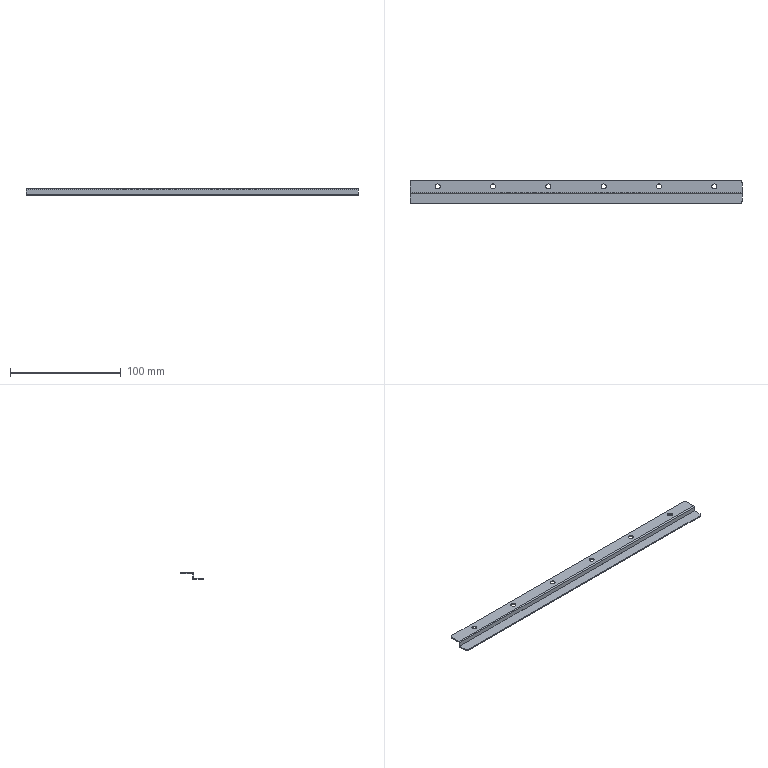Part | STEP file | Face cover reinforcing rib 300mm | 1 solid | 38 faces | box 300 x 21 x 6 mm | volume 7570 mm3 | cylinder 20 | plane 18 | commonest cylinder face diameters 4.5 x12 4 x4 0.02 x2 2.02 x2